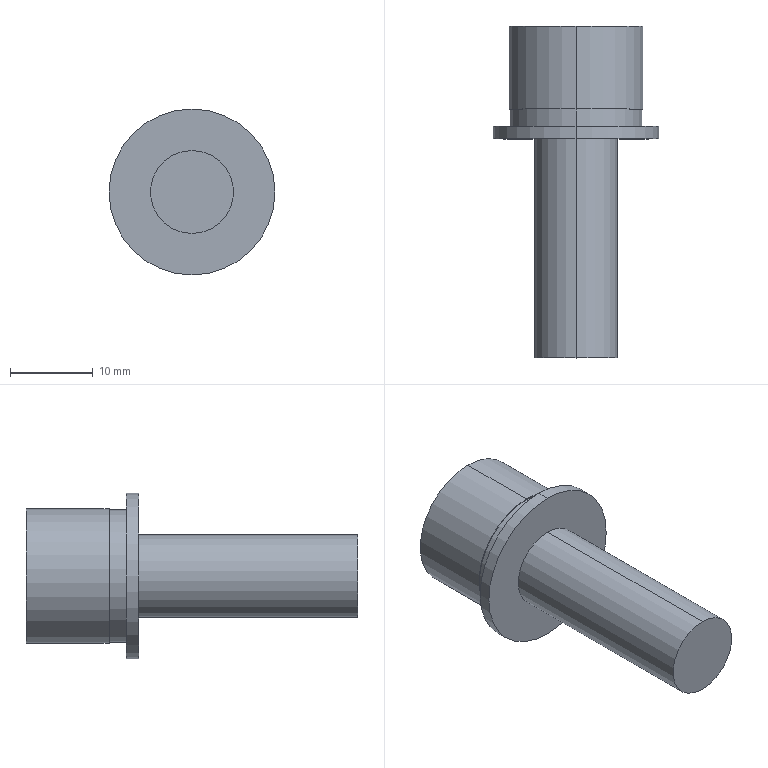Part | SolidWorks | features ICE 3, Revolution 1 | 3 solids | 26 faces | box 20 x 40 x 20 mm | volume 4696 mm3 | plane 14 | cylinder 12 | commonest cylinder face diameters 10 x6 16 x2 16.2 x2 20 x2
STEP:
#1=CARTESIAN_POINT('',(0.,-30.,5.));
#2=VERTEX_POINT('',#1);
#3=CARTESIAN_POINT('',(0.,-30.,-5.));
#4=VERTEX_POINT('',#3);
#5=CARTESIAN_POINT('',(0.,-30.,0.));
#6=DIRECTION('',(0.,1.,0.));
#7=DIRECTION('',(0.,0.,1.));
#8=AXIS2_PLACEMENT_3D('',#5,#6,#7);
#9=CIRCLE('',#8,5.);
#10=EDGE_CURVE('',#2,#4,#9,.T.);
#11=ORIENTED_EDGE('',*,*,#10,.T.);
#12=CARTESIAN_POINT('',(0.,0.,-5.));
#13=VERTEX_POINT('',#12);
#14=CARTESIAN_POINT('',(0.,11.322,-5.));
#15=DIRECTION('',(0.,1.,0.));
#16=VECTOR('',#15,1000.);
#17=LINE('',#14,#16);
#18=EDGE_CURVE('',#4,#13,#17,.T.);
#19=ORIENTED_EDGE('',*,*,#18,.T.);
#20=CARTESIAN_POINT('',(0.,0.,5.));
#21=VERTEX_POINT('',#20);
#22=CARTESIAN_POINT('',(0.,0.,0.));
#23=DIRECTION('',(0.,1.,0.));
#24=DIRECTION('',(0.,0.,1.));
#25=AXIS2_PLACEMENT_3D('',#22,#23,#24);
#26=CIRCLE('',#25,5.);
#27=EDGE_CURVE('',#21,#13,#26,.T.);
#28=ORIENTED_EDGE('',*,*,#27,.F.);
#29=CARTESIAN_POINT('',(0.,11.322,5.));
#30=DIRECTION('',(0.,1.,0.));
#31=VECTOR('',#30,1000.);
#32=LINE('',#29,#31);
#33=EDGE_CURVE('',#2,#21,#32,.T.);
#34=ORIENTED_EDGE('',*,*,#33,.F.);
#35=EDGE_LOOP('',(#11,#19,#28,#34));
#36=FACE_OUTER_BOUND('',#35,.T.);
#37=CARTESIAN_POINT('',(0.,11.322,0.));
#38=DIRECTION('',(0.,1.,0.));
#39=DIRECTION('',(0.,0.,1.));
#40=AXIS2_PLACEMENT_3D('',#37,#38,#39);
#41=CYLINDRICAL_SURFACE('',#40,5.);
#42=ADVANCED_FACE('',(#36),#41,.T.);
#43=CARTESIAN_POINT('',(0.,0.,8.1));
#44=VERTEX_POINT('',#43);
#45=CARTESIAN_POINT('',(0.,0.,-8.1));
#46=VERTEX_POINT('',#45);
#47=CARTESIAN_POINT('',(0.,0.,0.));
#48=DIRECTION('',(0.,1.,0.));
#49=DIRECTION('',(0.,0.,1.));
#50=AXIS2_PLACEMENT_3D('',#47,#48,#49);
#51=CIRCLE('',#50,8.1);
#52=EDGE_CURVE('',#44,#46,#51,.T.);
#53=ORIENTED_EDGE('',*,*,#52,.T.);
#54=CARTESIAN_POINT('',(0.,10.,-8.1));
#55=VERTEX_POINT('',#54);
#56=CARTESIAN_POINT('',(0.,11.322,-8.1));
#57=DIRECTION('',(0.,1.,0.));
#58=VECTOR('',#57,1000.);
#59=LINE('',#56,#58);
#60=EDGE_CURVE('',#46,#55,#59,.T.);
#61=ORIENTED_EDGE('',*,*,#60,.T.);
#62=CARTESIAN_POINT('',(0.,10.,8.1));
#63=VERTEX_POINT('',#62);
#64=CARTESIAN_POINT('',(0.,10.,0.));
#65=DIRECTION('',(0.,1.,0.));
#66=DIRECTION('',(0.,0.,1.));
#67=AXIS2_PLACEMENT_3D('',#64,#65,#66);
#68=CIRCLE('',#67,8.1);
#69=EDGE_CURVE('',#63,#55,#68,.T.);
#70=ORIENTED_EDGE('',*,*,#69,.F.);
#71=CARTESIAN_POINT('',(0.,11.322,8.1));
#72=DIRECTION('',(0.,1.,0.));
#73=VECTOR('',#72,1000.);
#74=LINE('',#71,#73);
#75=EDGE_CURVE('',#44,#63,#74,.T.);
#76=ORIENTED_EDGE('',*,*,#75,.F.);
#77=EDGE_LOOP('',(#53,#61,#70,#76));
#78=FACE_OUTER_BOUND('',#77,.T.);
#79=CARTESIAN_POINT('',(0.,11.322,0.));
#80=DIRECTION('',(0.,1.,0.));
#81=DIRECTION('',(0.,0.,1.));
#82=AXIS2_PLACEMENT_3D('',#79,#80,#81);
#83=CYLINDRICAL_SURFACE('',#82,8.1);
#84=ADVANCED_FACE('',(#78),#83,.T.);
#85=CARTESIAN_POINT('',(4.,10.,-2.309));
#86=VERTEX_POINT('',#85);
#87=CARTESIAN_POINT('',(0.,10.,-4.619));
#88=VERTEX_POINT('',#87);
#89=CARTESIAN_POINT('',(4.,10.,-2.309));
#90=DIRECTION('',(-0.866,0.,-0.5));
#91=VECTOR('',#90,1000.);
#92=LINE('',#89,#91);
#93=EDGE_CURVE('',#86,#88,#92,.T.);
#94=ORIENTED_EDGE('',*,*,#93,.F.);
#95=CARTESIAN_POINT('',(4.,10.,2.309));
#96=VERTEX_POINT('',#95);
#97=CARTESIAN_POINT('',(4.,10.,2.309));
#98=DIRECTION('',(0.,0.,-1.));
#99=VECTOR('',#98,1000.);
#100=LINE('',#97,#99);
#101=EDGE_CURVE('',#96,#86,#100,.T.);
#102=ORIENTED_EDGE('',*,*,#101,.F.);
#103=CARTESIAN_POINT('',(0.,10.,4.619));
#104=VERTEX_POINT('',#103);
#105=CARTESIAN_POINT('',(0.,10.,4.619));
#106=DIRECTION('',(0.866,0.,-0.5));
#107=VECTOR('',#106,1000.);
#108=LINE('',#105,#107);
#109=EDGE_CURVE('',#104,#96,#108,.T.);
#110=ORIENTED_EDGE('',*,*,#109,.F.);
#111=CARTESIAN_POINT('',(-4.,10.,2.309));
#112=VERTEX_POINT('',#111);
#113=CARTESIAN_POINT('',(-4.,10.,2.309));
#114=DIRECTION('',(0.866,0.,0.5));
#115=VECTOR('',#114,1000.);
#116=LINE('',#113,#115);
#117=EDGE_CURVE('',#112,#104,#116,.T.);
#118=ORIENTED_EDGE('',*,*,#117,.F.);
#119=CARTESIAN_POINT('',(-4.,10.,-2.309));
#120=VERTEX_POINT('',#119);
#121=CARTESIAN_POINT('',(-4.,10.,-2.309));
#122=DIRECTION('',(0.,0.,1.));
#123=VECTOR('',#122,1000.);
#124=LINE('',#121,#123);
#125=EDGE_CURVE('',#120,#112,#124,.T.);
#126=ORIENTED_EDGE('',*,*,#125,.F.);
#127=CARTESIAN_POINT('',(0.,10.,-4.619));
#128=DIRECTION('',(-0.866,0.,0.5));
#129=VECTOR('',#128,1000.);
#130=LINE('',#127,#129);
#131=EDGE_CURVE('',#88,#120,#130,.T.);
#132=ORIENTED_EDGE('',*,*,#131,.F.);
#133=EDGE_LOOP('',(#94,#102,#110,#118,#126,#132));
#134=FACE_BOUND('',#133,.T.);
#135=ORIENTED_EDGE('',*,*,#69,.T.);
#136=CARTESIAN_POINT('',(0.,10.,0.));
#137=DIRECTION('',(0.,1.,0.));
#138=DIRECTION('',(0.,0.,1.));
#139=AXIS2_PLACEMENT_3D('',#136,#137,#138);
#140=CIRCLE('',#139,8.1);
#141=EDGE_CURVE('',#55,#63,#140,.T.);
#142=ORIENTED_EDGE('',*,*,#141,.T.);
#143=EDGE_LOOP('',(#135,#142));
#144=FACE_OUTER_BOUND('',#143,.T.);
#145=CARTESIAN_POINT('',(0.,10.,0.));
#146=DIRECTION('',(0.,1.,0.));
#147=DIRECTION('',(0.,0.,1.));
#148=AXIS2_PLACEMENT_3D('',#145,#146,#147);
#149=PLANE('',#148);
#150=ADVANCED_FACE('',(#134,#144),#149,.T.);
#151=ORIENTED_EDGE('',*,*,#60,.F.);
#152=CARTESIAN_POINT('',(0.,0.,0.));
#153=DIRECTION('',(0.,1.,0.));
#154=DIRECTION('',(0.,0.,1.));
#155=AXIS2_PLACEMENT_3D('',#152,#153,#154);
#156=CIRCLE('',#155,8.1);
#157=EDGE_CURVE('',#46,#44,#156,.T.);
#158=ORIENTED_EDGE('',*,*,#157,.T.);
#159=ORIENTED_EDGE('',*,*,#75,.T.);
#160=ORIENTED_EDGE('',*,*,#141,.F.);
#161=EDGE_LOOP('',(#151,#158,#159,#160));
#162=FACE_OUTER_BOUND('',#161,.T.);
#163=CARTESIAN_POINT('',(0.,11.322,0.));
#164=DIRECTION('',(0.,1.,0.));
#165=DIRECTION('',(0.,0.,1.));
#166=AXIS2_PLACEMENT_3D('',#163,#164,#165);
#167=CYLINDRICAL_SURFACE('',#166,8.1);
#168=ADVANCED_FACE('',(#162),#167,.T.);
#169=ORIENTED_EDGE('',*,*,#27,.T.);
#170=CARTESIAN_POINT('',(0.,0.,0.));
#171=DIRECTION('',(0.,1.,0.));
#172=DIRECTION('',(0.,0.,1.));
#173=AXIS2_PLACEMENT_3D('',#170,#171,#172);
#174=CIRCLE('',#173,5.);
#175=EDGE_CURVE('',#13,#21,#174,.T.);
#176=ORIENTED_EDGE('',*,*,#175,.T.);
#177=EDGE_LOOP('',(#169,#176));
#178=FACE_BOUND('',#177,.T.);
#179=ORIENTED_EDGE('',*,*,#52,.F.);
#180=ORIENTED_EDGE('',*,*,#157,.F.);
#181=EDGE_LOOP('',(#179,#180));
#182=FACE_OUTER_BOUND('',#181,.T.);
#183=CARTESIAN_POINT('',(-8.1,0.,0.));
#184=DIRECTION('',(0.,-1.,0.));
#185=DIRECTION('',(0.,0.,-1.));
#186=AXIS2_PLACEMENT_3D('',#183,#184,#185);
#187=PLANE('',#186);
#188=ADVANCED_FACE('',(#178,#182),#187,.T.);
#189=ORIENTED_EDGE('',*,*,#18,.F.);
#190=CARTESIAN_POINT('',(0.,-30.,0.));
#191=DIRECTION('',(0.,1.,0.));
#192=DIRECTION('',(0.,0.,1.));
#193=AXIS2_PLACEMENT_3D('',#190,#191,#192);
#194=CIRCLE('',#193,5.);
#195=EDGE_CURVE('',#4,#2,#194,.T.);
#196=ORIENTED_EDGE('',*,*,#195,.T.);
#197=ORIENTED_EDGE('',*,*,#33,.T.);
#198=ORIENTED_EDGE('',*,*,#175,.F.);
#199=EDGE_LOOP('',(#189,#196,#197,#198));
#200=FACE_OUTER_BOUND('',#199,.T.);
#201=CARTESIAN_POINT('',(0.,11.322,0.));
#202=DIRECTION('',(0.,1.,0.));
#203=DIRECTION('',(0.,0.,1.));
#204=AXIS2_PLACEMENT_3D('',#201,#202,#203);
#205=CYLINDRICAL_SURFACE('',#204,5.);
#206=ADVANCED_FACE('',(#200),#205,.T.);
#207=ORIENTED_EDGE('',*,*,#10,.F.);
#208=ORIENTED_EDGE('',*,*,#195,.F.);
#209=EDGE_LOOP('',(#207,#208));
#210=FACE_OUTER_BOUND('',#209,.T.);
#211=CARTESIAN_POINT('',(-5.,-30.,0.));
#212=DIRECTION('',(0.,-1.,0.));
#213=DIRECTION('',(0.,0.,-1.));
#214=AXIS2_PLACEMENT_3D('',#211,#212,#213);
#215=PLANE('',#214);
#216=ADVANCED_FACE('',(#210),#215,.T.);
#217=ORIENTED_EDGE('',*,*,#93,.T.);
#218=CARTESIAN_POINT('',(0.,4.,-4.619));
#219=VERTEX_POINT('',#218);
#220=CARTESIAN_POINT('',(0.,4.,-4.619));
#221=DIRECTION('',(0.,1.,0.));
#222=VECTOR('',#221,1000.);
#223=LINE('',#220,#222);
#224=EDGE_CURVE('',#219,#88,#223,.T.);
#225=ORIENTED_EDGE('',*,*,#224,.F.);
#226=CARTESIAN_POINT('',(4.,4.,-2.309));
#227=VERTEX_POINT('',#226);
#228=CARTESIAN_POINT('',(4.,4.,-2.309));
#229=DIRECTION('',(-0.866,0.,-0.5));
#230=VECTOR('',#229,1000.);
#231=LINE('',#228,#230);
#232=EDGE_CURVE('',#227,#219,#231,.T.);
#233=ORIENTED_EDGE('',*,*,#232,.F.);
#234=CARTESIAN_POINT('',(4.,4.,-2.309));
#235=DIRECTION('',(0.,1.,0.));
#236=VECTOR('',#235,1000.);
#237=LINE('',#234,#236);
#238=EDGE_CURVE('',#227,#86,#237,.T.);
#239=ORIENTED_EDGE('',*,*,#238,.T.);
#240=EDGE_LOOP('',(#217,#225,#233,#239));
#241=FACE_OUTER_BOUND('',#240,.T.);
#242=CARTESIAN_POINT('',(4.,4.,-2.309));
#243=DIRECTION('',(0.5,0.,-0.866));
#244=DIRECTION('',(-0.866,0.,-0.5));
#245=AXIS2_PLACEMENT_3D('',#242,#243,#244);
#246=PLANE('',#245);
#247=ADVANCED_FACE('',(#241),#246,.F.);
#248=ORIENTED_EDGE('',*,*,#101,.T.);
#249=ORIENTED_EDGE('',*,*,#238,.F.);
#250=CARTESIAN_POINT('',(4.,4.,2.309));
#251=VERTEX_POINT('',#250);
#252=CARTESIAN_POINT('',(4.,4.,2.309));
#253=DIRECTION('',(0.,0.,-1.));
#254=VECTOR('',#253,1000.);
#255=LINE('',#252,#254);
#256=EDGE_CURVE('',#251,#227,#255,.T.);
#257=ORIENTED_EDGE('',*,*,#256,.F.);
#258=CARTESIAN_POINT('',(4.,4.,2.309));
#259=DIRECTION('',(0.,1.,0.));
#260=VECTOR('',#259,1000.);
#261=LINE('',#258,#260);
#262=EDGE_CURVE('',#251,#96,#261,.T.);
#263=ORIENTED_EDGE('',*,*,#262,.T.);
#264=EDGE_LOOP('',(#248,#249,#257,#263));
#265=FACE_OUTER_BOUND('',#264,.T.);
#266=CARTESIAN_POINT('',(4.,4.,2.309));
#267=DIRECTION('',(1.,0.,0.));
#268=DIRECTION('',(0.,0.,-1.));
#269=AXIS2_PLACEMENT_3D('',#266,#267,#268);
#270=PLANE('',#269);
#271=ADVANCED_FACE('',(#265),#270,.F.);
#272=ORIENTED_EDGE('',*,*,#109,.T.);
#273=ORIENTED_EDGE('',*,*,#262,.F.);
#274=CARTESIAN_POINT('',(0.,4.,4.619));
#275=VERTEX_POINT('',#274);
#276=CARTESIAN_POINT('',(0.,4.,4.619));
#277=DIRECTION('',(0.866,0.,-0.5));
#278=VECTOR('',#277,1000.);
#279=LINE('',#276,#278);
#280=EDGE_CURVE('',#275,#251,#279,.T.);
#281=ORIENTED_EDGE('',*,*,#280,.F.);
#282=CARTESIAN_POINT('',(0.,4.,4.619));
#283=DIRECTION('',(0.,1.,0.));
#284=VECTOR('',#283,1000.);
#285=LINE('',#282,#284);
#286=EDGE_CURVE('',#275,#104,#285,.T.);
#287=ORIENTED_EDGE('',*,*,#286,.T.);
#288=EDGE_LOOP('',(#272,#273,#281,#287));
#289=FACE_OUTER_BOUND('',#288,.T.);
#290=CARTESIAN_POINT('',(0.,4.,4.619));
#291=DIRECTION('',(0.5,0.,0.866));
#292=DIRECTION('',(0.866,0.,-0.5));
#293=AXIS2_PLACEMENT_3D('',#290,#291,#292);
#294=PLANE('',#293);
#295=ADVANCED_FACE('',(#289),#294,.F.);
#296=ORIENTED_EDGE('',*,*,#117,.T.);
#297=ORIENTED_EDGE('',*,*,#286,.F.);
#298=CARTESIAN_POINT('',(-4.,4.,2.309));
#299=VERTEX_POINT('',#298);
#300=CARTESIAN_POINT('',(-4.,4.,2.309));
#301=DIRECTION('',(0.866,0.,0.5));
#302=VECTOR('',#301,1000.);
#303=LINE('',#300,#302);
#304=EDGE_CURVE('',#299,#275,#303,.T.);
#305=ORIENTED_EDGE('',*,*,#304,.F.);
#306=CARTESIAN_POINT('',(-4.,4.,2.309));
#307=DIRECTION('',(0.,1.,0.));
#308=VECTOR('',#307,1000.);
#309=LINE('',#306,#308);
#310=EDGE_CURVE('',#299,#112,#309,.T.);
#311=ORIENTED_EDGE('',*,*,#310,.T.);
#312=EDGE_LOOP('',(#296,#297,#305,#311));
#313=FACE_OUTER_BOUND('',#312,.T.);
#314=CARTESIAN_POINT('',(-4.,4.,2.309));
#315=DIRECTION('',(-0.5,0.,0.866));
#316=DIRECTION('',(0.866,0.,0.5));
#317=AXIS2_PLACEMENT_3D('',#314,#315,#316);
#318=PLANE('',#317);
#319=ADVANCED_FACE('',(#313),#318,.F.);
#320=ORIENTED_EDGE('',*,*,#125,.T.);
#321=ORIENTED_EDGE('',*,*,#310,.F.);
#322=CARTESIAN_POINT('',(-4.,4.,-2.309));
#323=VERTEX_POINT('',#322);
#324=CARTESIAN_POINT('',(-4.,4.,-2.309));
#325=DIRECTION('',(0.,0.,1.));
#326=VECTOR('',#325,1000.);
#327=LINE('',#324,#326);
#328=EDGE_CURVE('',#323,#299,#327,.T.);
#329=ORIENTED_EDGE('',*,*,#328,.F.);
#330=CARTESIAN_POINT('',(-4.,4.,-2.309));
#331=DIRECTION('',(0.,1.,0.));
#332=VECTOR('',#331,1000.);
#333=LINE('',#330,#332);
#334=EDGE_CURVE('',#323,#120,#333,.T.);
#335=ORIENTED_EDGE('',*,*,#334,.T.);
#336=EDGE_LOOP('',(#320,#321,#329,#335));
#337=FACE_OUTER_BOUND('',#336,.T.);
#338=CARTESIAN_POINT('',(-4.,4.,-2.309));
#339=DIRECTION('',(-1.,0.,0.));
#340=DIRECTION('',(0.,0.,1.));
#341=AXIS2_PLACEMENT_3D('',#338,#339,#340);
#342=PLANE('',#341);
#343=ADVANCED_FACE('',(#337),#342,.F.);
#344=ORIENTED_EDGE('',*,*,#131,.T.);
#345=ORIENTED_EDGE('',*,*,#334,.F.);
#346=CARTESIAN_POINT('',(0.,4.,-4.619));
#347=DIRECTION('',(-0.866,0.,0.5));
#348=VECTOR('',#347,1000.);
#349=LINE('',#346,#348);
#350=EDGE_CURVE('',#219,#323,#349,.T.);
#351=ORIENTED_EDGE('',*,*,#350,.F.);
#352=ORIENTED_EDGE('',*,*,#224,.T.);
#353=EDGE_LOOP('',(#344,#345,#351,#352));
#354=FACE_OUTER_BOUND('',#353,.T.);
#355=CARTESIAN_POINT('',(0.,4.,-4.619));
#356=DIRECTION('',(-0.5,0.,-0.866));
#357=DIRECTION('',(-0.866,0.,0.5));
#358=AXIS2_PLACEMENT_3D('',#355,#356,#357);
#359=PLANE('',#358);
#360=ADVANCED_FACE('',(#354),#359,.F.);
#361=ORIENTED_EDGE('',*,*,#232,.T.);
#362=ORIENTED_EDGE('',*,*,#350,.T.);
#363=ORIENTED_EDGE('',*,*,#328,.T.);
#364=ORIENTED_EDGE('',*,*,#304,.T.);
#365=ORIENTED_EDGE('',*,*,#280,.T.);
#366=ORIENTED_EDGE('',*,*,#256,.T.);
#367=EDGE_LOOP('',(#361,#362,#363,#364,#365,#366));
#368=FACE_OUTER_BOUND('',#367,.T.);
#369=CARTESIAN_POINT('',(0.,4.,0.));
#370=DIRECTION('',(0.,1.,0.));
#371=DIRECTION('',(0.,0.,1.));
#372=AXIS2_PLACEMENT_3D('',#369,#370,#371);
#373=PLANE('',#372);
#374=ADVANCED_FACE('',(#368),#373,.T.);
#375=CLOSED_SHELL('',(#42,#84,#150,#168,#188,#206,#216,#247,#271,#295,#319,#343,#360,#374));
#376=MANIFOLD_SOLID_BREP('',#375);
#377=CARTESIAN_POINT('',(0.,-2.1,5.));
#378=VERTEX_POINT('',#377);
#379=CARTESIAN_POINT('',(0.,-2.1,-5.));
#380=VERTEX_POINT('',#379);
#381=CARTESIAN_POINT('',(0.,-2.1,0.));
#382=DIRECTION('',(0.,-1.,0.));
#383=DIRECTION('',(0.,0.,-1.));
#384=AXIS2_PLACEMENT_3D('',#381,#382,#383);
#385=CIRCLE('',#384,5.);
#386=EDGE_CURVE('',#378,#380,#385,.T.);
#387=ORIENTED_EDGE('',*,*,#386,.T.);
#388=CARTESIAN_POINT('',(0.,0.,-5.));
#389=VERTEX_POINT('',#388);
#390=CARTESIAN_POINT('',(0.,-2.1,-5.));
#391=DIRECTION('',(0.,1.,0.));
#392=VECTOR('',#391,1000.);
#393=LINE('',#390,#392);
#394=EDGE_CURVE('',#380,#389,#393,.T.);
#395=ORIENTED_EDGE('',*,*,#394,.T.);
#396=CARTESIAN_POINT('',(0.,0.,5.));
#397=VERTEX_POINT('',#396);
#398=CARTESIAN_POINT('',(0.,0.,0.));
#399=DIRECTION('',(0.,-1.,0.));
#400=DIRECTION('',(0.,0.,-1.));
#401=AXIS2_PLACEMENT_3D('',#398,#399,#400);
#402=CIRCLE('',#401,5.);
#403=EDGE_CURVE('',#397,#389,#402,.T.);
#404=ORIENTED_EDGE('',*,*,#403,.F.);
#405=CARTESIAN_POINT('',(0.,-2.1,5.));
#406=DIRECTION('',(0.,1.,0.));
#407=VECTOR('',#406,1000.);
#408=LINE('',#405,#407);
#409=EDGE_CURVE('',#378,#397,#408,.T.);
#410=ORIENTED_EDGE('',*,*,#409,.F.);
#411=EDGE_LOOP('',(#387,#395,#404,#410));
#412=FACE_OUTER_BOUND('',#411,.T.);
#413=CARTESIAN_POINT('',(0.,-2.1,0.));
#414=DIRECTION('',(0.,1.,0.));
#415=DIRECTION('',(0.,0.,1.));
#416=AXIS2_PLACEMENT_3D('',#413,#414,#415);
#417=CYLINDRICAL_SURFACE('',#416,5.);
#418=ADVANCED_FACE('',(#412),#417,.F.);
#419=CARTESIAN_POINT('',(0.,-2.1,-8.));
#420=VERTEX_POINT('',#419);
#421=CARTESIAN_POINT('',(0.,-2.1,8.));
#422=VERTEX_POINT('',#421);
#423=CARTESIAN_POINT('',(0.,-2.1,0.));
#424=DIRECTION('',(0.,-1.,0.));
#425=DIRECTION('',(0.,0.,-1.));
#426=AXIS2_PLACEMENT_3D('',#423,#424,#425);
#427=CIRCLE('',#426,8.);
#428=EDGE_CURVE('',#420,#422,#427,.T.);
#429=ORIENTED_EDGE('',*,*,#428,.F.);
#430=CARTESIAN_POINT('',(0.,0.,-8.));
#431=VERTEX_POINT('',#430);
#432=CARTESIAN_POINT('',(0.,-2.1,-8.));
#433=DIRECTION('',(0.,1.,0.));
#434=VECTOR('',#433,1000.);
#435=LINE('',#432,#434);
#436=EDGE_CURVE('',#420,#431,#435,.T.);
#437=ORIENTED_EDGE('',*,*,#436,.T.);
#438=CARTESIAN_POINT('',(0.,0.,8.));
#439=VERTEX_POINT('',#438);
#440=CARTESIAN_POINT('',(0.,0.,0.));
#441=DIRECTION('',(0.,-1.,0.));
#442=DIRECTION('',(0.,0.,-1.));
#443=AXIS2_PLACEMENT_3D('',#440,#441,#442);
#444=CIRCLE('',#443,8.);
#445=EDGE_CURVE('',#431,#439,#444,.T.);
#446=ORIENTED_EDGE('',*,*,#445,.T.);
#447=CARTESIAN_POINT('',(0.,-2.1,8.));
#448=DIRECTION('',(0.,1.,0.));
#449=VECTOR('',#448,1000.);
#450=LINE('',#447,#449);
#451=EDGE_CURVE('',#422,#439,#450,.T.);
#452=ORIENTED_EDGE('',*,*,#451,.F.);
#453=EDGE_LOOP('',(#429,#437,#446,#452));
#454=FACE_OUTER_BOUND('',#453,.T.);
#455=CARTESIAN_POINT('',(0.,-2.1,0.));
#456=DIRECTION('',(0.,1.,0.));
#457=DIRECTION('',(0.,0.,1.));
#458=AXIS2_PLACEMENT_3D('',#455,#456,#457);
#459=CYLINDRICAL_SURFACE('',#458,8.);
#460=ADVANCED_FACE('',(#454),#459,.T.);
#461=CARTESIAN_POINT('',(0.,-2.1,0.));
#462=DIRECTION('',(0.,-1.,0.));
#463=DIRECTION('',(0.,0.,-1.));
#464=AXIS2_PLACEMENT_3D('',#461,#462,#463);
#465=CIRCLE('',#464,8.);
#466=EDGE_CURVE('',#422,#420,#465,.T.);
#467=ORIENTED_EDGE('',*,*,#466,.T.);
#468=ORIENTED_EDGE('',*,*,#428,.T.);
#469=EDGE_LOOP('',(#467,#468));
#470=FACE_OUTER_BOUND('',#469,.T.);
#471=ORIENTED_EDGE('',*,*,#386,.F.);
#472=CARTESIAN_POINT('',(0.,-2.1,0.));
#473=DIRECTION('',(0.,-1.,0.));
#474=DIRECTION('',(0.,0.,-1.));
#475=AXIS2_PLACEMENT_3D('',#472,#473,#474);
#476=CIRCLE('',#475,5.);
#477=EDGE_CURVE('',#380,#378,#476,.T.);
#478=ORIENTED_EDGE('',*,*,#477,.F.);
#479=EDGE_LOOP('',(#471,#478));
#480=FACE_BOUND('',#479,.T.);
#481=CARTESIAN_POINT('',(0.,-2.1,0.));
#482=DIRECTION('',(0.,-1.,0.));
#483=DIRECTION('',(0.,0.,-1.));
#484=AXIS2_PLACEMENT_3D('',#481,#482,#483);
#485=PLANE('',#484);
#486=ADVANCED_FACE('',(#470,#480),#485,.T.);
#487=CARTESIAN_POINT('',(0.,0.,0.));
#488=DIRECTION('',(0.,-1.,0.));
#489=DIRECTION('',(0.,0.,-1.));
#490=AXIS2_PLACEMENT_3D('',#487,#488,#489);
#491=CIRCLE('',#490,8.);
#492=EDGE_CURVE('',#439,#431,#491,.T.);
#493=ORIENTED_EDGE('',*,*,#492,.F.);
#494=ORIENTED_EDGE('',*,*,#445,.F.);
#495=EDGE_LOOP('',(#493,#494));
#496=FACE_OUTER_BOUND('',#495,.T.);
#497=ORIENTED_EDGE('',*,*,#403,.T.);
#498=CARTESIAN_POINT('',(0.,0.,0.));
#499=DIRECTION('',(0.,-1.,0.));
#500=DIRECTION('',(0.,0.,-1.));
#501=AXIS2_PLACEMENT_3D('',#498,#499,#500);
#502=CIRCLE('',#501,5.);
#503=EDGE_CURVE('',#389,#397,#502,.T.);
#504=ORIENTED_EDGE('',*,*,#503,.T.);
#505=EDGE_LOOP('',(#497,#504));
#506=FACE_BOUND('',#505,.T.);
#507=CARTESIAN_POINT('',(0.,0.,0.));
#508=DIRECTION('',(0.,-1.,0.));
#509=DIRECTION('',(0.,0.,-1.));
#510=AXIS2_PLACEMENT_3D('',#507,#508,#509);
#511=PLANE('',#510);
#512=ADVANCED_FACE('',(#496,#506),#511,.F.);
#513=ORIENTED_EDGE('',*,*,#436,.F.);
#514=ORIENTED_EDGE('',*,*,#466,.F.);
#515=ORIENTED_EDGE('',*,*,#451,.T.);
#516=ORIENTED_EDGE('',*,*,#492,.T.);
#517=EDGE_LOOP('',(#513,#514,#515,#516));
#518=FACE_OUTER_BOUND('',#517,.T.);
#519=CARTESIAN_POINT('',(0.,-2.1,0.));
#520=DIRECTION('',(0.,1.,0.));
#521=DIRECTION('',(0.,0.,1.));
#522=AXIS2_PLACEMENT_3D('',#519,#520,#521);
#523=CYLINDRICAL_SURFACE('',#522,8.);
#524=ADVANCED_FACE('',(#518),#523,.T.);
#525=ORIENTED_EDGE('',*,*,#394,.F.);
#526=ORIENTED_EDGE('',*,*,#477,.T.);
#527=ORIENTED_EDGE('',*,*,#409,.T.);
#528=ORIENTED_EDGE('',*,*,#503,.F.);
#529=EDGE_LOOP('',(#525,#526,#527,#528));
#530=FACE_OUTER_BOUND('',#529,.T.);
#531=CARTESIAN_POINT('',(0.,-2.1,0.));
#532=DIRECTION('',(0.,1.,0.));
#533=DIRECTION('',(0.,0.,1.));
#534=AXIS2_PLACEMENT_3D('',#531,#532,#533);
#535=CYLINDRICAL_SURFACE('',#534,5.);
#536=ADVANCED_FACE('',(#530),#535,.F.);
#537=CLOSED_SHELL('',(#418,#460,#486,#512,#524,#536));
#538=MANIFOLD_SOLID_BREP('',#537);
#539=CARTESIAN_POINT('',(0.,-3.6,5.));
#540=VERTEX_POINT('',#539);
#541=CARTESIAN_POINT('',(0.,-3.6,-5.));
#542=VERTEX_POINT('',#541);
#543=CARTESIAN_POINT('',(0.,-3.6,0.));
#544=DIRECTION('',(0.,-1.,0.));
#545=DIRECTION('',(0.,0.,-1.));
#546=AXIS2_PLACEMENT_3D('',#543,#544,#545);
#547=CIRCLE('',#546,5.);
#548=EDGE_CURVE('',#540,#542,#547,.T.);
#549=ORIENTED_EDGE('',*,*,#548,.T.);
#550=CARTESIAN_POINT('',(0.,-2.1,-5.));
#551=VERTEX_POINT('',#550);
#552=CARTESIAN_POINT('',(0.,-3.6,-5.));
#553=DIRECTION('',(0.,1.,0.));
#554=VECTOR('',#553,1000.);
#555=LINE('',#552,#554);
#556=EDGE_CURVE('',#542,#551,#555,.T.);
#557=ORIENTED_EDGE('',*,*,#556,.T.);
#558=CARTESIAN_POINT('',(0.,-2.1,5.));
#559=VERTEX_POINT('',#558);
#560=CARTESIAN_POINT('',(0.,-2.1,0.));
#561=DIRECTION('',(0.,-1.,0.));
#562=DIRECTION('',(0.,0.,-1.));
#563=AXIS2_PLACEMENT_3D('',#560,#561,#562);
#564=CIRCLE('',#563,5.);
#565=EDGE_CURVE('',#559,#551,#564,.T.);
#566=ORIENTED_EDGE('',*,*,#565,.F.);
#567=CARTESIAN_POINT('',(0.,-3.6,5.));
#568=DIRECTION('',(0.,1.,0.));
#569=VECTOR('',#568,1000.);
#570=LINE('',#567,#569);
#571=EDGE_CURVE('',#540,#559,#570,.T.);
#572=ORIENTED_EDGE('',*,*,#571,.F.);
#573=EDGE_LOOP('',(#549,#557,#566,#572));
#574=FACE_OUTER_BOUND('',#573,.T.);
#575=CARTESIAN_POINT('',(0.,-3.6,0.));
#576=DIRECTION('',(0.,1.,0.));
#577=DIRECTION('',(0.,0.,1.));
#578=AXIS2_PLACEMENT_3D('',#575,#576,#577);
#579=CYLINDRICAL_SURFACE('',#578,5.);
#580=ADVANCED_FACE('',(#574),#579,.F.);
#581=CARTESIAN_POINT('',(0.,-3.6,-10.));
#582=VERTEX_POINT('',#581);
#583=CARTESIAN_POINT('',(0.,-3.6,10.));
#584=VERTEX_POINT('',#583);
#585=CARTESIAN_POINT('',(0.,-3.6,0.));
#586=DIRECTION('',(0.,-1.,0.));
#587=DIRECTION('',(0.,0.,-1.));
#588=AXIS2_PLACEMENT_3D('',#585,#586,#587);
#589=CIRCLE('',#588,10.);
#590=EDGE_CURVE('',#582,#584,#589,.T.);
#591=ORIENTED_EDGE('',*,*,#590,.F.);
#592=CARTESIAN_POINT('',(0.,-2.1,-10.));
#593=VERTEX_POINT('',#592);
#594=CARTESIAN_POINT('',(0.,-3.6,-10.));
#595=DIRECTION('',(0.,1.,0.));
#596=VECTOR('',#595,1000.);
#597=LINE('',#594,#596);
#598=EDGE_CURVE('',#582,#593,#597,.T.);
#599=ORIENTED_EDGE('',*,*,#598,.T.);
#600=CARTESIAN_POINT('',(0.,-2.1,10.));
#601=VERTEX_POINT('',#600);
#602=CARTESIAN_POINT('',(0.,-2.1,0.));
#603=DIRECTION('',(0.,-1.,0.));
#604=DIRECTION('',(0.,0.,-1.));
#605=AXIS2_PLACEMENT_3D('',#602,#603,#604);
#606=CIRCLE('',#605,10.);
#607=EDGE_CURVE('',#593,#601,#606,.T.);
#608=ORIENTED_EDGE('',*,*,#607,.T.);
#609=CARTESIAN_POINT('',(0.,-3.6,10.));
#610=DIRECTION('',(0.,1.,0.));
#611=VECTOR('',#610,1000.);
#612=LINE('',#609,#611);
#613=EDGE_CURVE('',#584,#601,#612,.T.);
#614=ORIENTED_EDGE('',*,*,#613,.F.);
#615=EDGE_LOOP('',(#591,#599,#608,#614));
#616=FACE_OUTER_BOUND('',#615,.T.);
#617=CARTESIAN_POINT('',(0.,-3.6,0.));
#618=DIRECTION('',(0.,1.,0.));
#619=DIRECTION('',(0.,0.,1.));
#620=AXIS2_PLACEMENT_3D('',#617,#618,#619);
#621=CYLINDRICAL_SURFACE('',#620,10.);
#622=ADVANCED_FACE('',(#616),#621,.T.);
#623=CARTESIAN_POINT('',(0.,-3.6,0.));
#624=DIRECTION('',(0.,-1.,0.));
#625=DIRECTION('',(0.,0.,-1.));
#626=AXIS2_PLACEMENT_3D('',#623,#624,#625);
#627=CIRCLE('',#626,10.);
#628=EDGE_CURVE('',#584,#582,#627,.T.);
#629=ORIENTED_EDGE('',*,*,#628,.T.);
#630=ORIENTED_EDGE('',*,*,#590,.T.);
#631=EDGE_LOOP('',(#629,#630));
#632=FACE_OUTER_BOUND('',#631,.T.);
#633=ORIENTED_EDGE('',*,*,#548,.F.);
#634=CARTESIAN_POINT('',(0.,-3.6,0.));
#635=DIRECTION('',(0.,-1.,0.));
#636=DIRECTION('',(0.,0.,-1.));
#637=AXIS2_PLACEMENT_3D('',#634,#635,#636);
#638=CIRCLE('',#637,5.);
#639=EDGE_CURVE('',#542,#540,#638,.T.);
#640=ORIENTED_EDGE('',*,*,#639,.F.);
#641=EDGE_LOOP('',(#633,#640));
#642=FACE_BOUND('',#641,.T.);
#643=CARTESIAN_POINT('',(0.,-3.6,0.));
#644=DIRECTION('',(0.,-1.,0.));
#645=DIRECTION('',(0.,0.,-1.));
#646=AXIS2_PLACEMENT_3D('',#643,#644,#645);
#647=PLANE('',#646);
#648=ADVANCED_FACE('',(#632,#642),#647,.T.);
#649=CARTESIAN_POINT('',(0.,-2.1,0.));
#650=DIRECTION('',(0.,-1.,0.));
#651=DIRECTION('',(0.,0.,-1.));
#652=AXIS2_PLACEMENT_3D('',#649,#650,#651);
#653=CIRCLE('',#652,10.);
#654=EDGE_CURVE('',#601,#593,#653,.T.);
#655=ORIENTED_EDGE('',*,*,#654,.F.);
#656=ORIENTED_EDGE('',*,*,#607,.F.);
#657=EDGE_LOOP('',(#655,#656));
#658=FACE_OUTER_BOUND('',#657,.T.);
#659=ORIENTED_EDGE('',*,*,#565,.T.);
#660=CARTESIAN_POINT('',(0.,-2.1,0.));
#661=DIRECTION('',(0.,-1.,0.));
#662=DIRECTION('',(0.,0.,-1.));
#663=AXIS2_PLACEMENT_3D('',#660,#661,#662);
#664=CIRCLE('',#663,5.);
#665=EDGE_CURVE('',#551,#559,#664,.T.);
#666=ORIENTED_EDGE('',*,*,#665,.T.);
#667=EDGE_LOOP('',(#659,#666));
#668=FACE_BOUND('',#667,.T.);
#669=CARTESIAN_POINT('',(0.,-2.1,0.));
#670=DIRECTION('',(0.,-1.,0.));
#671=DIRECTION('',(0.,0.,-1.));
#672=AXIS2_PLACEMENT_3D('',#669,#670,#671);
#673=PLANE('',#672);
#674=ADVANCED_FACE('',(#658,#668),#673,.F.);
#675=ORIENTED_EDGE('',*,*,#598,.F.);
#676=ORIENTED_EDGE('',*,*,#628,.F.);
#677=ORIENTED_EDGE('',*,*,#613,.T.);
#678=ORIENTED_EDGE('',*,*,#654,.T.);
#679=EDGE_LOOP('',(#675,#676,#677,#678));
#680=FACE_OUTER_BOUND('',#679,.T.);
#681=CARTESIAN_POINT('',(0.,-3.6,0.));
#682=DIRECTION('',(0.,1.,0.));
#683=DIRECTION('',(0.,0.,1.));
#684=AXIS2_PLACEMENT_3D('',#681,#682,#683);
#685=CYLINDRICAL_SURFACE('',#684,10.);
#686=ADVANCED_FACE('',(#680),#685,.T.);
#687=ORIENTED_EDGE('',*,*,#556,.F.);
#688=ORIENTED_EDGE('',*,*,#639,.T.);
#689=ORIENTED_EDGE('',*,*,#571,.T.);
#690=ORIENTED_EDGE('',*,*,#665,.F.);
#691=EDGE_LOOP('',(#687,#688,#689,#690));
#692=FACE_OUTER_BOUND('',#691,.T.);
#693=CARTESIAN_POINT('',(0.,-3.6,0.));
#694=DIRECTION('',(0.,1.,0.));
#695=DIRECTION('',(0.,0.,1.));
#696=AXIS2_PLACEMENT_3D('',#693,#694,#695);
#697=CYLINDRICAL_SURFACE('',#696,5.);
#698=ADVANCED_FACE('',(#692),#697,.F.);
#699=CLOSED_SHELL('',(#580,#622,#648,#674,#686,#698));
#700=MANIFOLD_SOLID_BREP('',#699);
#701=CARTESIAN_POINT('',(0.,0.,0.));
#702=DIRECTION('',(0.,0.,1.));
#703=DIRECTION('',(1.,0.,0.));
#704=AXIS2_PLACEMENT_3D('',#701,#702,#703);
#705=(LENGTH_UNIT()NAMED_UNIT(*)SI_UNIT(.MILLI.,.METRE.));
#706=UNCERTAINTY_MEASURE_WITH_UNIT(LENGTH_MEASURE(0.00001),#705,'','');
#707=(NAMED_UNIT(*)PLANE_ANGLE_UNIT()SI_UNIT($,.RADIAN.));
#708=(NAMED_UNIT(*)SI_UNIT($,.STERADIAN.)SOLID_ANGLE_UNIT());
#709=(GEOMETRIC_REPRESENTATION_CONTEXT(3)GLOBAL_UNCERTAINTY_ASSIGNED_CONTEXT((#706))GLOBAL_UNIT_ASSIGNED_CONTEXT((#705,#707,#708))REPRESENTATION_CONTEXT('',''));
#710=ADVANCED_BREP_SHAPE_REPRESENTATION('',(#376,#538,#700,#704),#709);